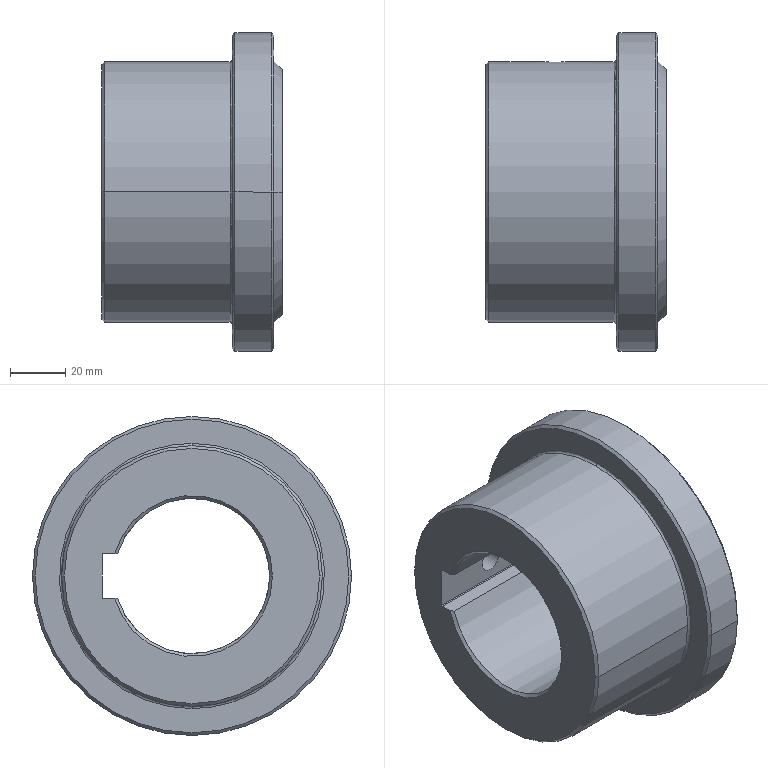Part | SolidWorks | features BaseBody 1 | 1 solid | 29 faces | box 65 x 115 x 115 mm | volume 335130 mm3 | cone 11 | cylinder 9 | plane 7 | spline 2 | commonest cylinder face diameters 0.5 x2 8.376 x2 94 x2 115 x2 56 x1